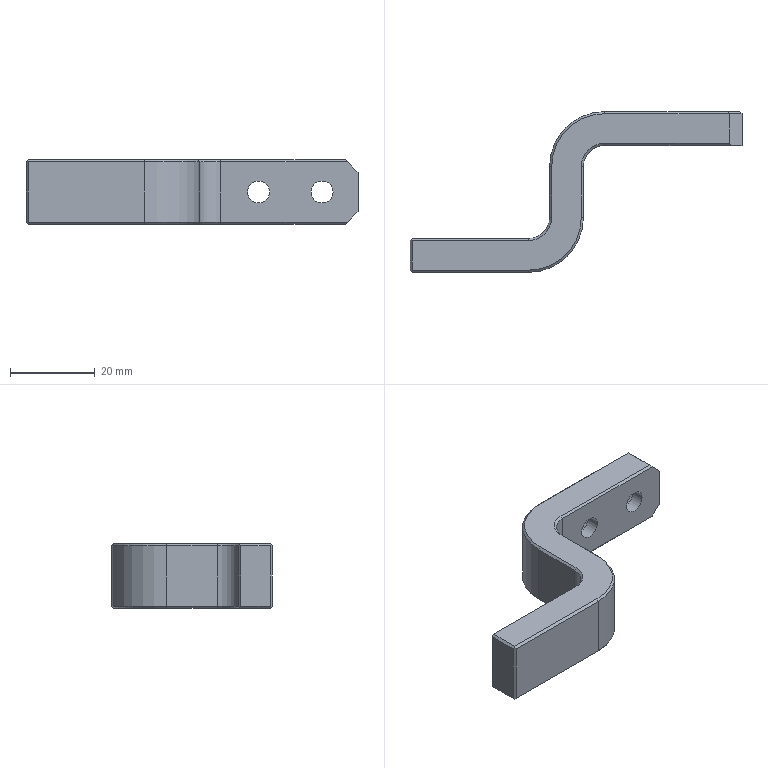Part | Creo | features CURVE 3, DATUM PLANE 3, CHAMFER 2, CUT 2, COORDINATE SYSTEM 1, PROTRUSION 1 | 1 solid | 53 faces | box 78.5 x 38 x 15.3 mm | volume 11414 mm3 | plane 33 | cylinder 12 | cone 8 | commonest cylinder face diameters 5.2 x4 9.2 x4 10 x2 26 x2
STEP:
#1=CARTESIAN_POINT('',(0.,0.,0.));
#2=DIRECTION('',(0.,0.,1.));
#3=DIRECTION('',(1.,0.,0.));
#4=AXIS2_PLACEMENT_3D('',#1,#2,#3);
#5=CARTESIAN_POINT('',(25.5,7.5,-7.65));
#6=VERTEX_POINT('',#5);
#7=CARTESIAN_POINT('',(-4.,7.5,-7.65));
#8=VERTEX_POINT('',#7);
#9=CARTESIAN_POINT('',(25.5,7.5,-7.65));
#10=DIRECTION('',(-1.,0.,0.));
#11=VECTOR('',#10,29.5);
#12=LINE('',#9,#11);
#13=EDGE_CURVE('',#6,#8,#12,.T.);
#14=ORIENTED_EDGE('',*,*,#13,.F.);
#15=CARTESIAN_POINT('',(25.5,14.5,-7.65));
#16=VERTEX_POINT('',#15);
#17=CARTESIAN_POINT('',(25.5,14.5,-7.65));
#18=DIRECTION('',(0.,-1.,0.));
#19=VECTOR('',#18,7.);
#20=LINE('',#17,#19);
#21=EDGE_CURVE('',#16,#6,#20,.T.);
#22=ORIENTED_EDGE('',*,*,#21,.F.);
#23=CARTESIAN_POINT('',(-4.,14.5,-7.65));
#24=VERTEX_POINT('',#23);
#25=CARTESIAN_POINT('',(-4.,14.5,-7.65));
#26=DIRECTION('',(1.,0.,0.));
#27=VECTOR('',#26,29.5);
#28=LINE('',#25,#27);
#29=EDGE_CURVE('',#24,#16,#28,.T.);
#30=ORIENTED_EDGE('',*,*,#29,.F.);
#31=CARTESIAN_POINT('',(-16.5,2.,-7.65));
#32=VERTEX_POINT('',#31);
#33=CARTESIAN_POINT('',(-4.,2.,-7.65));
#34=DIRECTION('',(0.,0.,-1.));
#35=DIRECTION('',(-1.,0.,0.));
#36=AXIS2_PLACEMENT_3D('',#33,#34,#35);
#37=CIRCLE('',#36,12.5);
#38=EDGE_CURVE('',#32,#24,#37,.T.);
#39=ORIENTED_EDGE('',*,*,#38,.F.);
#40=CARTESIAN_POINT('',(-16.5,-10.,-7.65));
#41=VERTEX_POINT('',#40);
#42=CARTESIAN_POINT('',(-16.5,-10.,-7.65));
#43=DIRECTION('',(0.,1.,0.));
#44=VECTOR('',#43,12.);
#45=LINE('',#42,#44);
#46=EDGE_CURVE('',#41,#32,#45,.T.);
#47=ORIENTED_EDGE('',*,*,#46,.F.);
#48=CARTESIAN_POINT('',(-22.,-15.5,-7.65));
#49=VERTEX_POINT('',#48);
#50=CARTESIAN_POINT('',(-22.,-10.,-7.65));
#51=DIRECTION('',(0.,0.,1.));
#52=DIRECTION('',(0.,-1.,0.));
#53=AXIS2_PLACEMENT_3D('',#50,#51,#52);
#54=CIRCLE('',#53,5.5);
#55=EDGE_CURVE('',#49,#41,#54,.T.);
#56=ORIENTED_EDGE('',*,*,#55,.F.);
#57=CARTESIAN_POINT('',(-49.5,-15.5,-7.65));
#58=VERTEX_POINT('',#57);
#59=CARTESIAN_POINT('',(-49.5,-15.5,-7.65));
#60=DIRECTION('',(1.,0.,0.));
#61=VECTOR('',#60,27.5);
#62=LINE('',#59,#61);
#63=EDGE_CURVE('',#58,#49,#62,.T.);
#64=ORIENTED_EDGE('',*,*,#63,.F.);
#65=CARTESIAN_POINT('',(-49.5,-22.5,-7.65));
#66=VERTEX_POINT('',#65);
#67=CARTESIAN_POINT('',(-49.5,-22.5,-7.65));
#68=DIRECTION('',(0.,1.,0.));
#69=VECTOR('',#68,7.);
#70=LINE('',#67,#69);
#71=EDGE_CURVE('',#66,#58,#70,.T.);
#72=ORIENTED_EDGE('',*,*,#71,.F.);
#73=CARTESIAN_POINT('',(-22.,-22.5,-7.65));
#74=VERTEX_POINT('',#73);
#75=CARTESIAN_POINT('',(-22.,-22.5,-7.65));
#76=DIRECTION('',(-1.,0.,0.));
#77=VECTOR('',#76,27.5);
#78=LINE('',#75,#77);
#79=EDGE_CURVE('',#74,#66,#78,.T.);
#80=ORIENTED_EDGE('',*,*,#79,.F.);
#81=CARTESIAN_POINT('',(-9.5,-10.,-7.65));
#82=VERTEX_POINT('',#81);
#83=CARTESIAN_POINT('',(-22.,-10.,-7.65));
#84=DIRECTION('',(0.,0.,-1.));
#85=DIRECTION('',(1.,0.,0.));
#86=AXIS2_PLACEMENT_3D('',#83,#84,#85);
#87=CIRCLE('',#86,12.5);
#88=EDGE_CURVE('',#82,#74,#87,.T.);
#89=ORIENTED_EDGE('',*,*,#88,.F.);
#90=CARTESIAN_POINT('',(-9.5,2.,-7.65));
#91=VERTEX_POINT('',#90);
#92=CARTESIAN_POINT('',(-9.5,2.,-7.65));
#93=DIRECTION('',(0.,-1.,0.));
#94=VECTOR('',#93,12.);
#95=LINE('',#92,#94);
#96=EDGE_CURVE('',#91,#82,#95,.T.);
#97=ORIENTED_EDGE('',*,*,#96,.F.);
#98=CARTESIAN_POINT('',(-4.,2.,-7.65));
#99=DIRECTION('',(0.,0.,1.));
#100=DIRECTION('',(0.,1.,0.));
#101=AXIS2_PLACEMENT_3D('',#98,#99,#100);
#102=CIRCLE('',#101,5.5);
#103=EDGE_CURVE('',#8,#91,#102,.T.);
#104=ORIENTED_EDGE('',*,*,#103,.F.);
#105=EDGE_LOOP('',(#14,#22,#30,#39,#47,#56,#64,#72,#80,#89,#97,#104));
#106=FACE_OUTER_BOUND('',#105,.F.);
#107=CARTESIAN_POINT('',(0.,0.,-7.65));
#108=DIRECTION('',(0.,0.,1.));
#109=DIRECTION('',(1.,0.,0.));
#110=AXIS2_PLACEMENT_3D('',#107,#108,#109);
#111=PLANE('',#110);
#112=ADVANCED_FACE('',(#106),#111,.F.);
#113=CARTESIAN_POINT('',(26.,7.,-7.15));
#114=VERTEX_POINT('',#113);
#115=CARTESIAN_POINT('',(26.,7.,-7.15));
#116=DIRECTION('',(-0.5774,0.5774,-0.5774));
#117=VECTOR('',#116,0.866);
#118=LINE('',#115,#117);
#119=EDGE_CURVE('',#114,#6,#118,.T.);
#120=ORIENTED_EDGE('',*,*,#119,.T.);
#121=ORIENTED_EDGE('',*,*,#13,.T.);
#122=CARTESIAN_POINT('',(-4.,7.,-7.15));
#123=VERTEX_POINT('',#122);
#124=CARTESIAN_POINT('',(-4.,7.5,-7.65));
#125=DIRECTION('',(0.000000027,-0.7071,0.7071));
#126=VECTOR('',#125,0.7071);
#127=LINE('',#124,#126);
#128=EDGE_CURVE('',#8,#123,#127,.T.);
#129=ORIENTED_EDGE('',*,*,#128,.T.);
#130=CARTESIAN_POINT('',(26.,7.,-7.15));
#131=DIRECTION('',(-1.,0.,0.));
#132=VECTOR('',#131,30.);
#133=LINE('',#130,#132);
#134=EDGE_CURVE('',#114,#123,#133,.T.);
#135=ORIENTED_EDGE('',*,*,#134,.F.);
#136=EDGE_LOOP('',(#120,#121,#129,#135));
#137=FACE_OUTER_BOUND('',#136,.F.);
#138=CARTESIAN_POINT('',(10.75,7.25,-7.4));
#139=DIRECTION('',(0.,-0.7071,-0.7071));
#140=DIRECTION('',(0.,-0.7071,0.7071));
#141=AXIS2_PLACEMENT_3D('',#138,#139,#140);
#142=PLANE('',#141);
#143=ADVANCED_FACE('',(#137),#142,.T.);
#144=ORIENTED_EDGE('',*,*,#119,.F.);
#145=CARTESIAN_POINT('',(28.5,7.,-4.65));
#146=VERTEX_POINT('',#145);
#147=CARTESIAN_POINT('',(26.,7.,-7.15));
#148=DIRECTION('',(0.7071,0.,0.7071));
#149=VECTOR('',#148,3.536);
#150=LINE('',#147,#149);
#151=EDGE_CURVE('',#114,#146,#150,.T.);
#152=ORIENTED_EDGE('',*,*,#151,.T.);
#153=CARTESIAN_POINT('',(28.5,14.5,-4.65));
#154=VERTEX_POINT('',#153);
#155=CARTESIAN_POINT('',(28.5,14.5,-4.65));
#156=DIRECTION('',(0.,-1.,0.));
#157=VECTOR('',#156,7.5);
#158=LINE('',#155,#157);
#159=EDGE_CURVE('',#154,#146,#158,.T.);
#160=ORIENTED_EDGE('',*,*,#159,.F.);
#161=CARTESIAN_POINT('',(28.5,14.5,-4.65));
#162=DIRECTION('',(-0.7071,0.,-0.7071));
#163=VECTOR('',#162,4.243);
#164=LINE('',#161,#163);
#165=EDGE_CURVE('',#154,#16,#164,.T.);
#166=ORIENTED_EDGE('',*,*,#165,.T.);
#167=ORIENTED_EDGE('',*,*,#21,.T.);
#168=EDGE_LOOP('',(#144,#152,#160,#166,#167));
#169=FACE_OUTER_BOUND('',#168,.F.);
#170=CARTESIAN_POINT('',(27.,11.,-6.15));
#171=DIRECTION('',(0.7071,0.,-0.7071));
#172=DIRECTION('',(0.7071,0.,0.7071));
#173=AXIS2_PLACEMENT_3D('',#170,#171,#172);
#174=PLANE('',#173);
#175=ADVANCED_FACE('',(#169),#174,.T.);
#176=CARTESIAN_POINT('',(-4.,7.,7.15));
#177=VERTEX_POINT('',#176);
#178=CARTESIAN_POINT('',(26.,7.,7.15));
#179=VERTEX_POINT('',#178);
#180=CARTESIAN_POINT('',(-4.,7.,7.15));
#181=DIRECTION('',(1.,0.,0.));
#182=VECTOR('',#181,30.);
#183=LINE('',#180,#182);
#184=EDGE_CURVE('',#177,#179,#183,.T.);
#185=ORIENTED_EDGE('',*,*,#184,.T.);
#186=CARTESIAN_POINT('',(28.5,7.,4.65));
#187=VERTEX_POINT('',#186);
#188=CARTESIAN_POINT('',(28.5,7.,4.65));
#189=DIRECTION('',(-0.7071,0.,0.7071));
#190=VECTOR('',#189,3.536);
#191=LINE('',#188,#190);
#192=EDGE_CURVE('',#187,#179,#191,.T.);
#193=ORIENTED_EDGE('',*,*,#192,.F.);
#194=CARTESIAN_POINT('',(28.5,7.,-4.65));
#195=DIRECTION('',(0.,0.,1.));
#196=VECTOR('',#195,9.3);
#197=LINE('',#194,#196);
#198=EDGE_CURVE('',#146,#187,#197,.T.);
#199=ORIENTED_EDGE('',*,*,#198,.F.);
#200=ORIENTED_EDGE('',*,*,#151,.F.);
#201=ORIENTED_EDGE('',*,*,#134,.T.);
#202=CARTESIAN_POINT('',(-4.,7.,-7.15));
#203=DIRECTION('',(-0.000000003,0.,1.));
#204=VECTOR('',#203,14.3);
#205=LINE('',#202,#204);
#206=EDGE_CURVE('',#123,#177,#205,.T.);
#207=ORIENTED_EDGE('',*,*,#206,.T.);
#208=EDGE_LOOP('',(#185,#193,#199,#200,#201,#207));
#209=FACE_OUTER_BOUND('',#208,.F.);
#210=CARTESIAN_POINT('',(7.6,7.,0.));
#211=VERTEX_POINT('',#210);
#212=CARTESIAN_POINT('',(2.4,7.,0.));
#213=VERTEX_POINT('',#212);
#214=CARTESIAN_POINT('',(5.,7.,0.));
#215=DIRECTION('',(0.,1.,0.));
#216=DIRECTION('',(1.,0.,0.));
#217=AXIS2_PLACEMENT_3D('',#214,#215,#216);
#218=CIRCLE('',#217,2.6);
#219=EDGE_CURVE('',#211,#213,#218,.T.);
#220=ORIENTED_EDGE('',*,*,#219,.F.);
#221=CARTESIAN_POINT('',(5.,7.,0.));
#222=DIRECTION('',(0.,1.,0.));
#223=DIRECTION('',(-1.,0.,0.));
#224=AXIS2_PLACEMENT_3D('',#221,#222,#223);
#225=CIRCLE('',#224,2.6);
#226=EDGE_CURVE('',#213,#211,#225,.T.);
#227=ORIENTED_EDGE('',*,*,#226,.F.);
#228=EDGE_LOOP('',(#220,#227));
#229=FACE_BOUND('',#228,.F.);
#230=CARTESIAN_POINT('',(22.6,7.,0.));
#231=VERTEX_POINT('',#230);
#232=CARTESIAN_POINT('',(17.4,7.,0.));
#233=VERTEX_POINT('',#232);
#234=CARTESIAN_POINT('',(20.,7.,0.));
#235=DIRECTION('',(0.,1.,0.));
#236=DIRECTION('',(1.,0.,0.));
#237=AXIS2_PLACEMENT_3D('',#234,#235,#236);
#238=CIRCLE('',#237,2.6);
#239=EDGE_CURVE('',#231,#233,#238,.T.);
#240=ORIENTED_EDGE('',*,*,#239,.F.);
#241=CARTESIAN_POINT('',(20.,7.,0.));
#242=DIRECTION('',(0.,1.,0.));
#243=DIRECTION('',(-1.,0.,0.));
#244=AXIS2_PLACEMENT_3D('',#241,#242,#243);
#245=CIRCLE('',#244,2.6);
#246=EDGE_CURVE('',#233,#231,#245,.T.);
#247=ORIENTED_EDGE('',*,*,#246,.F.);
#248=EDGE_LOOP('',(#240,#247));
#249=FACE_BOUND('',#248,.F.);
#250=CARTESIAN_POINT('',(-4.,7.,-7.65));
#251=DIRECTION('',(0.,-1.,0.));
#252=DIRECTION('',(1.,0.,0.));
#253=AXIS2_PLACEMENT_3D('',#250,#251,#252);
#254=PLANE('',#253);
#255=ADVANCED_FACE('',(#209,#229,#249),#254,.T.);
#256=CARTESIAN_POINT('',(22.6,10.,0.));
#257=VERTEX_POINT('',#256);
#258=CARTESIAN_POINT('',(17.4,10.,0.));
#259=VERTEX_POINT('',#258);
#260=CARTESIAN_POINT('',(20.,10.,0.));
#261=DIRECTION('',(0.,1.,0.));
#262=DIRECTION('',(1.,0.,0.));
#263=AXIS2_PLACEMENT_3D('',#260,#261,#262);
#264=CIRCLE('',#263,2.6);
#265=EDGE_CURVE('',#257,#259,#264,.T.);
#266=ORIENTED_EDGE('',*,*,#265,.F.);
#267=CARTESIAN_POINT('',(22.6,10.,0.));
#268=DIRECTION('',(0.,-1.,0.));
#269=VECTOR('',#268,3.);
#270=LINE('',#267,#269);
#271=EDGE_CURVE('',#257,#231,#270,.T.);
#272=ORIENTED_EDGE('',*,*,#271,.T.);
#273=ORIENTED_EDGE('',*,*,#239,.T.);
#274=CARTESIAN_POINT('',(17.4,10.,0.));
#275=DIRECTION('',(0.,-1.,0.));
#276=VECTOR('',#275,3.);
#277=LINE('',#274,#276);
#278=EDGE_CURVE('',#259,#233,#277,.T.);
#279=ORIENTED_EDGE('',*,*,#278,.F.);
#280=EDGE_LOOP('',(#266,#272,#273,#279));
#281=FACE_OUTER_BOUND('',#280,.F.);
#282=CARTESIAN_POINT('',(20.,15.,0.));
#283=DIRECTION('',(0.,1.,0.));
#284=DIRECTION('',(1.,0.,0.));
#285=AXIS2_PLACEMENT_3D('',#282,#283,#284);
#286=CYLINDRICAL_SURFACE('',#285,2.6);
#287=ADVANCED_FACE('',(#281),#286,.F.);
#288=CARTESIAN_POINT('',(24.6,10.,0.));
#289=VERTEX_POINT('',#288);
#290=CARTESIAN_POINT('',(15.4,10.,0.));
#291=VERTEX_POINT('',#290);
#292=CARTESIAN_POINT('',(20.,10.,0.));
#293=DIRECTION('',(0.,1.,0.));
#294=DIRECTION('',(1.,0.,0.));
#295=AXIS2_PLACEMENT_3D('',#292,#293,#294);
#296=CIRCLE('',#295,4.6);
#297=EDGE_CURVE('',#289,#291,#296,.T.);
#298=ORIENTED_EDGE('',*,*,#297,.F.);
#299=CARTESIAN_POINT('',(20.,10.,0.));
#300=DIRECTION('',(0.,1.,0.));
#301=DIRECTION('',(-1.,0.,0.));
#302=AXIS2_PLACEMENT_3D('',#299,#300,#301);
#303=CIRCLE('',#302,4.6);
#304=EDGE_CURVE('',#291,#289,#303,.T.);
#305=ORIENTED_EDGE('',*,*,#304,.F.);
#306=EDGE_LOOP('',(#298,#305));
#307=FACE_OUTER_BOUND('',#306,.F.);
#308=ORIENTED_EDGE('',*,*,#265,.T.);
#309=CARTESIAN_POINT('',(20.,10.,0.));
#310=DIRECTION('',(0.,1.,0.));
#311=DIRECTION('',(-1.,0.,0.));
#312=AXIS2_PLACEMENT_3D('',#309,#310,#311);
#313=CIRCLE('',#312,2.6);
#314=EDGE_CURVE('',#259,#257,#313,.T.);
#315=ORIENTED_EDGE('',*,*,#314,.T.);
#316=EDGE_LOOP('',(#308,#315));
#317=FACE_BOUND('',#316,.F.);
#318=CARTESIAN_POINT('',(0.,10.,-7.65));
#319=DIRECTION('',(0.,1.,0.));
#320=DIRECTION('',(1.,0.,0.));
#321=AXIS2_PLACEMENT_3D('',#318,#319,#320);
#322=PLANE('',#321);
#323=ADVANCED_FACE('',(#307,#317),#322,.T.);
#324=CARTESIAN_POINT('',(9.6,10.,0.));
#325=VERTEX_POINT('',#324);
#326=CARTESIAN_POINT('',(0.4,10.,0.));
#327=VERTEX_POINT('',#326);
#328=CARTESIAN_POINT('',(5.,10.,0.));
#329=DIRECTION('',(0.,1.,0.));
#330=DIRECTION('',(1.,0.,0.));
#331=AXIS2_PLACEMENT_3D('',#328,#329,#330);
#332=CIRCLE('',#331,4.6);
#333=EDGE_CURVE('',#325,#327,#332,.T.);
#334=ORIENTED_EDGE('',*,*,#333,.F.);
#335=CARTESIAN_POINT('',(5.,10.,0.));
#336=DIRECTION('',(0.,1.,0.));
#337=DIRECTION('',(-1.,0.,0.));
#338=AXIS2_PLACEMENT_3D('',#335,#336,#337);
#339=CIRCLE('',#338,4.6);
#340=EDGE_CURVE('',#327,#325,#339,.T.);
#341=ORIENTED_EDGE('',*,*,#340,.F.);
#342=EDGE_LOOP('',(#334,#341));
#343=FACE_OUTER_BOUND('',#342,.F.);
#344=CARTESIAN_POINT('',(7.6,10.,0.));
#345=VERTEX_POINT('',#344);
#346=CARTESIAN_POINT('',(2.4,10.,0.));
#347=VERTEX_POINT('',#346);
#348=CARTESIAN_POINT('',(5.,10.,0.));
#349=DIRECTION('',(0.,1.,0.));
#350=DIRECTION('',(1.,0.,0.));
#351=AXIS2_PLACEMENT_3D('',#348,#349,#350);
#352=CIRCLE('',#351,2.6);
#353=EDGE_CURVE('',#345,#347,#352,.T.);
#354=ORIENTED_EDGE('',*,*,#353,.T.);
#355=CARTESIAN_POINT('',(5.,10.,0.));
#356=DIRECTION('',(0.,1.,0.));
#357=DIRECTION('',(-1.,0.,0.));
#358=AXIS2_PLACEMENT_3D('',#355,#356,#357);
#359=CIRCLE('',#358,2.6);
#360=EDGE_CURVE('',#347,#345,#359,.T.);
#361=ORIENTED_EDGE('',*,*,#360,.T.);
#362=EDGE_LOOP('',(#354,#361));
#363=FACE_BOUND('',#362,.F.);
#364=CARTESIAN_POINT('',(0.,10.,-7.65));
#365=DIRECTION('',(0.,1.,0.));
#366=DIRECTION('',(1.,0.,0.));
#367=AXIS2_PLACEMENT_3D('',#364,#365,#366);
#368=PLANE('',#367);
#369=ADVANCED_FACE('',(#343,#363),#368,.T.);
#370=CARTESIAN_POINT('',(24.6,15.,0.));
#371=VERTEX_POINT('',#370);
#372=CARTESIAN_POINT('',(15.4,15.,0.));
#373=VERTEX_POINT('',#372);
#374=CARTESIAN_POINT('',(20.,15.,0.));
#375=DIRECTION('',(0.,1.,0.));
#376=DIRECTION('',(1.,0.,0.));
#377=AXIS2_PLACEMENT_3D('',#374,#375,#376);
#378=CIRCLE('',#377,4.6);
#379=EDGE_CURVE('',#371,#373,#378,.T.);
#380=ORIENTED_EDGE('',*,*,#379,.F.);
#381=CARTESIAN_POINT('',(24.6,15.,0.));
#382=DIRECTION('',(0.,-1.,0.));
#383=VECTOR('',#382,5.);
#384=LINE('',#381,#383);
#385=EDGE_CURVE('',#371,#289,#384,.T.);
#386=ORIENTED_EDGE('',*,*,#385,.T.);
#387=ORIENTED_EDGE('',*,*,#297,.T.);
#388=CARTESIAN_POINT('',(15.4,15.,0.));
#389=DIRECTION('',(0.,-1.,0.));
#390=VECTOR('',#389,5.);
#391=LINE('',#388,#390);
#392=EDGE_CURVE('',#373,#291,#391,.T.);
#393=ORIENTED_EDGE('',*,*,#392,.F.);
#394=EDGE_LOOP('',(#380,#386,#387,#393));
#395=FACE_OUTER_BOUND('',#394,.F.);
#396=CARTESIAN_POINT('',(20.,15.,0.));
#397=DIRECTION('',(0.,1.,0.));
#398=DIRECTION('',(1.,0.,0.));
#399=AXIS2_PLACEMENT_3D('',#396,#397,#398);
#400=CYLINDRICAL_SURFACE('',#399,4.6);
#401=ADVANCED_FACE('',(#395),#400,.F.);
#402=CARTESIAN_POINT('',(-4.,15.,-7.15));
#403=VERTEX_POINT('',#402);
#404=CARTESIAN_POINT('',(25.293,15.,-7.15));
#405=VERTEX_POINT('',#404);
#406=CARTESIAN_POINT('',(-4.,15.,-7.15));
#407=DIRECTION('',(1.,0.,0.));
#408=VECTOR('',#407,29.293);
#409=LINE('',#406,#408);
#410=EDGE_CURVE('',#403,#405,#409,.T.);
#411=ORIENTED_EDGE('',*,*,#410,.T.);
#412=CARTESIAN_POINT('',(28.,15.,-4.443));
#413=VERTEX_POINT('',#412);
#414=CARTESIAN_POINT('',(28.,15.,-4.443));
#415=DIRECTION('',(-0.7071,0.,-0.7071));
#416=VECTOR('',#415,3.828);
#417=LINE('',#414,#416);
#418=EDGE_CURVE('',#413,#405,#417,.T.);
#419=ORIENTED_EDGE('',*,*,#418,.F.);
#420=CARTESIAN_POINT('',(28.,15.,4.443));
#421=VERTEX_POINT('',#420);
#422=CARTESIAN_POINT('',(28.,15.,4.443));
#423=DIRECTION('',(0.,0.,-1.));
#424=VECTOR('',#423,8.886);
#425=LINE('',#422,#424);
#426=EDGE_CURVE('',#421,#413,#425,.T.);
#427=ORIENTED_EDGE('',*,*,#426,.F.);
#428=CARTESIAN_POINT('',(25.293,15.,7.15));
#429=VERTEX_POINT('',#428);
#430=CARTESIAN_POINT('',(25.293,15.,7.15));
#431=DIRECTION('',(0.7071,0.,-0.7071));
#432=VECTOR('',#431,3.828);
#433=LINE('',#430,#432);
#434=EDGE_CURVE('',#429,#421,#433,.T.);
#435=ORIENTED_EDGE('',*,*,#434,.F.);
#436=CARTESIAN_POINT('',(-4.,15.,7.15));
#437=VERTEX_POINT('',#436);
#438=CARTESIAN_POINT('',(25.293,15.,7.15));
#439=DIRECTION('',(-1.,0.,0.));
#440=VECTOR('',#439,29.293);
#441=LINE('',#438,#440);
#442=EDGE_CURVE('',#429,#437,#441,.T.);
#443=ORIENTED_EDGE('',*,*,#442,.T.);
#444=CARTESIAN_POINT('',(-4.,15.,-7.15));
#445=DIRECTION('',(0.000000002,0.,1.));
#446=VECTOR('',#445,14.3);
#447=LINE('',#444,#446);
#448=EDGE_CURVE('',#403,#437,#447,.T.);
#449=ORIENTED_EDGE('',*,*,#448,.F.);
#450=EDGE_LOOP('',(#411,#419,#427,#435,#443,#449));
#451=FACE_OUTER_BOUND('',#450,.F.);
#452=CARTESIAN_POINT('',(9.6,15.,0.));
#453=VERTEX_POINT('',#452);
#454=CARTESIAN_POINT('',(0.4,15.,0.));
#455=VERTEX_POINT('',#454);
#456=CARTESIAN_POINT('',(5.,15.,0.));
#457=DIRECTION('',(0.,1.,0.));
#458=DIRECTION('',(1.,0.,0.));
#459=AXIS2_PLACEMENT_3D('',#456,#457,#458);
#460=CIRCLE('',#459,4.6);
#461=EDGE_CURVE('',#453,#455,#460,.T.);
#462=ORIENTED_EDGE('',*,*,#461,.T.);
#463=CARTESIAN_POINT('',(5.,15.,0.));
#464=DIRECTION('',(0.,1.,0.));
#465=DIRECTION('',(-1.,0.,0.));
#466=AXIS2_PLACEMENT_3D('',#463,#464,#465);
#467=CIRCLE('',#466,4.6);
#468=EDGE_CURVE('',#455,#453,#467,.T.);
#469=ORIENTED_EDGE('',*,*,#468,.T.);
#470=EDGE_LOOP('',(#462,#469));
#471=FACE_BOUND('',#470,.F.);
#472=ORIENTED_EDGE('',*,*,#379,.T.);
#473=CARTESIAN_POINT('',(20.,15.,0.));
#474=DIRECTION('',(0.,1.,0.));
#475=DIRECTION('',(-1.,0.,0.));
#476=AXIS2_PLACEMENT_3D('',#473,#474,#475);
#477=CIRCLE('',#476,4.6);
#478=EDGE_CURVE('',#373,#371,#477,.T.);
#479=ORIENTED_EDGE('',*,*,#478,.T.);
#480=EDGE_LOOP('',(#472,#479));
#481=FACE_BOUND('',#480,.F.);
#482=CARTESIAN_POINT('',(28.5,15.,-7.65));
#483=DIRECTION('',(0.,1.,0.));
#484=DIRECTION('',(-1.,0.,0.));
#485=AXIS2_PLACEMENT_3D('',#482,#483,#484);
#486=PLANE('',#485);
#487=ADVANCED_FACE('',(#451,#471,#481),#486,.T.);
#488=ORIENTED_EDGE('',*,*,#478,.F.);
#489=ORIENTED_EDGE('',*,*,#392,.T.);
#490=ORIENTED_EDGE('',*,*,#304,.T.);
#491=ORIENTED_EDGE('',*,*,#385,.F.);
#492=EDGE_LOOP('',(#488,#489,#490,#491));
#493=FACE_OUTER_BOUND('',#492,.F.);
#494=CARTESIAN_POINT('',(20.,15.,0.));
#495=DIRECTION('',(0.,1.,0.));
#496=DIRECTION('',(1.,0.,0.));
#497=AXIS2_PLACEMENT_3D('',#494,#495,#496);
#498=CYLINDRICAL_SURFACE('',#497,4.6);
#499=ADVANCED_FACE('',(#493),#498,.F.);
#500=ORIENTED_EDGE('',*,*,#461,.F.);
#501=CARTESIAN_POINT('',(9.6,15.,0.));
#502=DIRECTION('',(0.,-1.,0.));
#503=VECTOR('',#502,5.);
#504=LINE('',#501,#503);
#505=EDGE_CURVE('',#453,#325,#504,.T.);
#506=ORIENTED_EDGE('',*,*,#505,.T.);
#507=ORIENTED_EDGE('',*,*,#333,.T.);
#508=CARTESIAN_POINT('',(0.4,15.,0.));
#509=DIRECTION('',(0.,-1.,0.));
#510=VECTOR('',#509,5.);
#511=LINE('',#508,#510);
#512=EDGE_CURVE('',#455,#327,#511,.T.);
#513=ORIENTED_EDGE('',*,*,#512,.F.);
#514=EDGE_LOOP('',(#500,#506,#507,#513));
#515=FACE_OUTER_BOUND('',#514,.F.);
#516=CARTESIAN_POINT('',(5.,15.,0.));
#517=DIRECTION('',(0.,1.,0.));
#518=DIRECTION('',(1.,0.,0.));
#519=AXIS2_PLACEMENT_3D('',#516,#517,#518);
#520=CYLINDRICAL_SURFACE('',#519,4.6);
#521=ADVANCED_FACE('',(#515),#520,.F.);
#522=ORIENTED_EDGE('',*,*,#468,.F.);
#523=ORIENTED_EDGE('',*,*,#512,.T.);
#524=ORIENTED_EDGE('',*,*,#340,.T.);
#525=ORIENTED_EDGE('',*,*,#505,.F.);
#526=EDGE_LOOP('',(#522,#523,#524,#525));
#527=FACE_OUTER_BOUND('',#526,.F.);
#528=CARTESIAN_POINT('',(5.,15.,0.));
#529=DIRECTION('',(0.,1.,0.));
#530=DIRECTION('',(1.,0.,0.));
#531=AXIS2_PLACEMENT_3D('',#528,#529,#530);
#532=CYLINDRICAL_SURFACE('',#531,4.6);
#533=ADVANCED_FACE('',(#527),#532,.F.);
#534=ORIENTED_EDGE('',*,*,#410,.F.);
#535=CARTESIAN_POINT('',(-4.,14.5,-7.65));
#536=DIRECTION('',(-0.000000009,0.7071,0.7071));
#537=VECTOR('',#536,0.7071);
#538=LINE('',#535,#537);
#539=EDGE_CURVE('',#24,#403,#538,.T.);
#540=ORIENTED_EDGE('',*,*,#539,.F.);
#541=ORIENTED_EDGE('',*,*,#29,.T.);
#542=CARTESIAN_POINT('',(25.5,14.5,-7.65));
#543=DIRECTION('',(-0.2811,0.6786,0.6786));
#544=VECTOR('',#543,0.7368);
#545=LINE('',#542,#544);
#546=EDGE_CURVE('',#16,#405,#545,.T.);
#547=ORIENTED_EDGE('',*,*,#546,.T.);
#548=EDGE_LOOP('',(#534,#540,#541,#547));
#549=FACE_OUTER_BOUND('',#548,.F.);
#550=CARTESIAN_POINT('',(10.75,14.75,-7.4));
#551=DIRECTION('',(0.,0.7071,-0.7071));
#552=DIRECTION('',(0.,0.7071,0.7071));
#553=AXIS2_PLACEMENT_3D('',#550,#551,#552);
#554=PLANE('',#553);
#555=ADVANCED_FACE('',(#549),#554,.T.);
#556=ORIENTED_EDGE('',*,*,#38,.T.);
#557=ORIENTED_EDGE('',*,*,#539,.T.);
#558=CARTESIAN_POINT('',(-17.,2.,-7.15));
#559=VERTEX_POINT('',#558);
#560=CARTESIAN_POINT('',(-4.,2.,-7.15));
#561=DIRECTION('',(0.,0.,-1.));
#562=DIRECTION('',(-1.,0.,0.));
#563=AXIS2_PLACEMENT_3D('',#560,#561,#562);
#564=CIRCLE('',#563,13.);
#565=EDGE_CURVE('',#559,#403,#564,.T.);
#566=ORIENTED_EDGE('',*,*,#565,.F.);
#567=CARTESIAN_POINT('',(-16.5,2.,-7.65));
#568=DIRECTION('',(-0.7071,0.00000001,0.7071));
#569=VECTOR('',#568,0.7071);
#570=LINE('',#567,#569);
#571=EDGE_CURVE('',#32,#559,#570,.T.);
#572=ORIENTED_EDGE('',*,*,#571,.F.);
#573=EDGE_LOOP('',(#556,#557,#566,#572));
#574=FACE_OUTER_BOUND('',#573,.F.);
#575=CARTESIAN_POINT('',(-4.,2.,-7.4));
#576=DIRECTION('',(0.,0.,1.));
#577=DIRECTION('',(0.,-1.,0.));
#578=AXIS2_PLACEMENT_3D('',#575,#576,#577);
#579=CONICAL_SURFACE('',#578,12.75,45.);
#580=ADVANCED_FACE('',(#574),#579,.T.);
#581=ORIENTED_EDGE('',*,*,#565,.T.);
#582=ORIENTED_EDGE('',*,*,#448,.T.);
#583=CARTESIAN_POINT('',(-17.,2.,7.15));
#584=VERTEX_POINT('',#583);
#585=CARTESIAN_POINT('',(-4.,2.,7.15));
#586=DIRECTION('',(0.,0.,1.));
#587=DIRECTION('',(0.,1.,0.));
#588=AXIS2_PLACEMENT_3D('',#585,#586,#587);
#589=CIRCLE('',#588,13.);
#590=EDGE_CURVE('',#437,#584,#589,.T.);
#591=ORIENTED_EDGE('',*,*,#590,.T.);
#592=CARTESIAN_POINT('',(-17.,2.,-7.15));
#593=DIRECTION('',(0.,0.,1.));
#594=VECTOR('',#593,14.3);
#595=LINE('',#592,#594);
#596=EDGE_CURVE('',#559,#584,#595,.T.);
#597=ORIENTED_EDGE('',*,*,#596,.F.);
#598=EDGE_LOOP('',(#581,#582,#591,#597));
#599=FACE_OUTER_BOUND('',#598,.F.);
#600=CARTESIAN_POINT('',(-4.,2.,-7.65));
#601=DIRECTION('',(0.,0.,1.));
#602=DIRECTION('',(1.,0.,0.));
#603=AXIS2_PLACEMENT_3D('',#600,#601,#602);
#604=CYLINDRICAL_SURFACE('',#603,13.);
#605=ADVANCED_FACE('',(#599),#604,.T.);
#606=CARTESIAN_POINT('',(-4.,14.5,7.65));
#607=VERTEX_POINT('',#606);
#608=CARTESIAN_POINT('',(-16.5,2.,7.65));
#609=VERTEX_POINT('',#608);
#610=CARTESIAN_POINT('',(-4.,2.,7.65));
#611=DIRECTION('',(0.,0.,1.));
#612=DIRECTION('',(0.,1.,0.));
#613=AXIS2_PLACEMENT_3D('',#610,#611,#612);
#614=CIRCLE('',#613,12.5);
#615=EDGE_CURVE('',#607,#609,#614,.T.);
#616=ORIENTED_EDGE('',*,*,#615,.T.);
#617=CARTESIAN_POINT('',(-16.5,2.,7.65));
#618=DIRECTION('',(-0.7071,0.00000001,-0.7071));
#619=VECTOR('',#618,0.7071);
#620=LINE('',#617,#619);
#621=EDGE_CURVE('',#609,#584,#620,.T.);
#622=ORIENTED_EDGE('',*,*,#621,.T.);
#623=ORIENTED_EDGE('',*,*,#590,.F.);
#624=CARTESIAN_POINT('',(-4.,14.5,7.65));
#625=DIRECTION('',(0.000000023,0.7071,-0.7071));
#626=VECTOR('',#625,0.7071);
#627=LINE('',#624,#626);
#628=EDGE_CURVE('',#607,#437,#627,.T.);
#629=ORIENTED_EDGE('',*,*,#628,.F.);
#630=EDGE_LOOP('',(#616,#622,#623,#629));
#631=FACE_OUTER_BOUND('',#630,.F.);
#632=CARTESIAN_POINT('',(-4.,2.,7.4));
#633=DIRECTION('',(0.,0.,-1.));
#634=DIRECTION('',(0.,-1.,0.));
#635=AXIS2_PLACEMENT_3D('',#632,#633,#634);
#636=CONICAL_SURFACE('',#635,12.75,45.);
#637=ADVANCED_FACE('',(#631),#636,.T.);
#638=CARTESIAN_POINT('',(-49.5,-15.5,7.65));
#639=VERTEX_POINT('',#638);
#640=CARTESIAN_POINT('',(-49.5,-22.5,7.65));
#641=VERTEX_POINT('',#640);
#642=CARTESIAN_POINT('',(-49.5,-15.5,7.65));
#643=DIRECTION('',(0.,-1.,0.));
#644=VECTOR('',#643,7.);
#645=LINE('',#642,#644);
#646=EDGE_CURVE('',#639,#641,#645,.T.);
#647=ORIENTED_EDGE('',*,*,#646,.F.);
#648=CARTESIAN_POINT('',(-22.,-15.5,7.65));
#649=VERTEX_POINT('',#648);
#650=CARTESIAN_POINT('',(-22.,-15.5,7.65));
#651=DIRECTION('',(-1.,0.,0.));
#652=VECTOR('',#651,27.5);
#653=LINE('',#650,#652);
#654=EDGE_CURVE('',#649,#639,#653,.T.);
#655=ORIENTED_EDGE('',*,*,#654,.F.);
#656=CARTESIAN_POINT('',(-16.5,-10.,7.65));
#657=VERTEX_POINT('',#656);
#658=CARTESIAN_POINT('',(-22.,-10.,7.65));
#659=DIRECTION('',(0.,0.,-1.));
#660=DIRECTION('',(1.,0.,0.));
#661=AXIS2_PLACEMENT_3D('',#658,#659,#660);
#662=CIRCLE('',#661,5.5);
#663=EDGE_CURVE('',#657,#649,#662,.T.);
#664=ORIENTED_EDGE('',*,*,#663,.F.);
#665=CARTESIAN_POINT('',(-16.5,2.,7.65));
#666=DIRECTION('',(0.,-1.,0.));
#667=VECTOR('',#666,12.);
#668=LINE('',#665,#667);
#669=EDGE_CURVE('',#609,#657,#668,.T.);
#670=ORIENTED_EDGE('',*,*,#669,.F.);
#671=ORIENTED_EDGE('',*,*,#615,.F.);
#672=CARTESIAN_POINT('',(25.5,14.5,7.65));
#673=VERTEX_POINT('',#672);
#674=CARTESIAN_POINT('',(25.5,14.5,7.65));
#675=DIRECTION('',(-1.,0.,0.));
#676=VECTOR('',#675,29.5);
#677=LINE('',#674,#676);
#678=EDGE_CURVE('',#673,#607,#677,.T.);
#679=ORIENTED_EDGE('',*,*,#678,.F.);
#680=CARTESIAN_POINT('',(25.5,7.5,7.65));
#681=VERTEX_POINT('',#680);
#682=CARTESIAN_POINT('',(25.5,7.5,7.65));
#683=DIRECTION('',(0.,1.,0.));
#684=VECTOR('',#683,7.);
#685=LINE('',#682,#684);
#686=EDGE_CURVE('',#681,#673,#685,.T.);
#687=ORIENTED_EDGE('',*,*,#686,.F.);
#688=CARTESIAN_POINT('',(-4.,7.5,7.65));
#689=VERTEX_POINT('',#688);
#690=CARTESIAN_POINT('',(-4.,7.5,7.65));
#691=DIRECTION('',(1.,0.,0.));
#692=VECTOR('',#691,29.5);
#693=LINE('',#690,#692);
#694=EDGE_CURVE('',#689,#681,#693,.T.);
#695=ORIENTED_EDGE('',*,*,#694,.F.);
#696=CARTESIAN_POINT('',(-9.5,2.,7.65));
#697=VERTEX_POINT('',#696);
#698=CARTESIAN_POINT('',(-4.,2.,7.65));
#699=DIRECTION('',(0.,0.,-1.));
#700=DIRECTION('',(-1.,0.,0.));
#701=AXIS2_PLACEMENT_3D('',#698,#699,#700);
#702=CIRCLE('',#701,5.5);
#703=EDGE_CURVE('',#697,#689,#702,.T.);
#704=ORIENTED_EDGE('',*,*,#703,.F.);
#705=CARTESIAN_POINT('',(-9.5,-10.,7.65));
#706=VERTEX_POINT('',#705);
#707=CARTESIAN_POINT('',(-9.5,-10.,7.65));
#708=DIRECTION('',(0.,1.,0.));
#709=VECTOR('',#708,12.);
#710=LINE('',#707,#709);
#711=EDGE_CURVE('',#706,#697,#710,.T.);
#712=ORIENTED_EDGE('',*,*,#711,.F.);
#713=CARTESIAN_POINT('',(-22.,-22.5,7.65));
#714=VERTEX_POINT('',#713);
#715=CARTESIAN_POINT('',(-22.,-10.,7.65));
#716=DIRECTION('',(0.,0.,1.));
#717=DIRECTION('',(0.,-1.,0.));
#718=AXIS2_PLACEMENT_3D('',#715,#716,#717);
#719=CIRCLE('',#718,12.5);
#720=EDGE_CURVE('',#714,#706,#719,.T.);
#721=ORIENTED_EDGE('',*,*,#720,.F.);
#722=CARTESIAN_POINT('',(-49.5,-22.5,7.65));
#723=DIRECTION('',(1.,0.,0.));
#724=VECTOR('',#723,27.5);
#725=LINE('',#722,#724);
#726=EDGE_CURVE('',#641,#714,#725,.T.);
#727=ORIENTED_EDGE('',*,*,#726,.F.);
#728=EDGE_LOOP('',(#647,#655,#664,#670,#671,#679,#687,#695,#704,#712,#721,#727));
#729=FACE_OUTER_BOUND('',#728,.F.);
#730=CARTESIAN_POINT('',(0.,0.,7.65));
#731=DIRECTION('',(0.,0.,1.));
#732=DIRECTION('',(1.,0.,0.));
#733=AXIS2_PLACEMENT_3D('',#730,#731,#732);
#734=PLANE('',#733);
#735=ADVANCED_FACE('',(#729),#734,.T.);
#736=CARTESIAN_POINT('',(-50.,-15.5,7.15));
#737=VERTEX_POINT('',#736);
#738=CARTESIAN_POINT('',(-50.,-22.5,7.15));
#739=VERTEX_POINT('',#738);
#740=CARTESIAN_POINT('',(-50.,-15.5,7.15));
#741=DIRECTION('',(0.,-1.,0.));
#742=VECTOR('',#741,7.);
#743=LINE('',#740,#742);
#744=EDGE_CURVE('',#737,#739,#743,.T.);
#745=ORIENTED_EDGE('',*,*,#744,.F.);
#746=CARTESIAN_POINT('',(-49.75,-15.25,7.4));
#747=VERTEX_POINT('',#746);
#748=CARTESIAN_POINT('',(-50.,-15.5,7.15));
#749=DIRECTION('',(0.5774,0.5774,0.5774));
#750=VECTOR('',#749,0.433);
#751=LINE('',#748,#750);
#752=EDGE_CURVE('',#737,#747,#751,.T.);
#753=ORIENTED_EDGE('',*,*,#752,.T.);
#754=CARTESIAN_POINT('',(-49.5,-15.5,7.65));
#755=DIRECTION('',(-0.5774,0.5774,-0.5774));
#756=VECTOR('',#755,0.433);
#757=LINE('',#754,#756);
#758=EDGE_CURVE('',#639,#747,#757,.T.);
#759=ORIENTED_EDGE('',*,*,#758,.F.);
#760=ORIENTED_EDGE('',*,*,#646,.T.);
#761=CARTESIAN_POINT('',(-49.75,-22.75,7.4));
#762=VERTEX_POINT('',#761);
#763=CARTESIAN_POINT('',(-49.5,-22.5,7.65));
#764=DIRECTION('',(-0.5774,-0.5774,-0.5774));
#765=VECTOR('',#764,0.433);
#766=LINE('',#763,#765);
#767=EDGE_CURVE('',#641,#762,#766,.T.);
#768=ORIENTED_EDGE('',*,*,#767,.T.);
#769=CARTESIAN_POINT('',(-49.75,-22.75,7.4));
#770=DIRECTION('',(-0.5774,0.5774,-0.5774));
#771=VECTOR('',#770,0.433);
#772=LINE('',#769,#771);
#773=EDGE_CURVE('',#762,#739,#772,.T.);
#774=ORIENTED_EDGE('',*,*,#773,.T.);
#775=EDGE_LOOP('',(#745,#753,#759,#760,#768,#774));
#776=FACE_OUTER_BOUND('',#775,.F.);
#777=CARTESIAN_POINT('',(-49.75,-19.,7.4));
#778=DIRECTION('',(-0.7071,0.,0.7071));
#779=DIRECTION('',(-0.7071,0.,-0.7071));
#780=AXIS2_PLACEMENT_3D('',#777,#778,#779);
#781=PLANE('',#780);
#782=ADVANCED_FACE('',(#776),#781,.T.);
#783=CARTESIAN_POINT('',(-50.,-15.5,-7.15));
#784=VERTEX_POINT('',#783);
#785=CARTESIAN_POINT('',(-50.,-15.5,7.15));
#786=DIRECTION('',(0.,0.,-1.));
#787=VECTOR('',#786,14.3);
#788=LINE('',#785,#787);
#789=EDGE_CURVE('',#737,#784,#788,.T.);
#790=ORIENTED_EDGE('',*,*,#789,.F.);
#791=ORIENTED_EDGE('',*,*,#744,.T.);
#792=CARTESIAN_POINT('',(-50.,-22.5,-7.15));
#793=VERTEX_POINT('',#792);
#794=CARTESIAN_POINT('',(-50.,-22.5,7.15));
#795=DIRECTION('',(0.,0.,-1.));
#796=VECTOR('',#795,14.3);
#797=LINE('',#794,#796);
#798=EDGE_CURVE('',#739,#793,#797,.T.);
#799=ORIENTED_EDGE('',*,*,#798,.T.);
#800=CARTESIAN_POINT('',(-50.,-22.5,-7.15));
#801=DIRECTION('',(0.,1.,0.));
#802=VECTOR('',#801,7.);
#803=LINE('',#800,#802);
#804=EDGE_CURVE('',#793,#784,#803,.T.);
#805=ORIENTED_EDGE('',*,*,#804,.T.);
#806=EDGE_LOOP('',(#790,#791,#799,#805));
#807=FACE_OUTER_BOUND('',#806,.F.);
#808=CARTESIAN_POINT('',(-50.,-15.,-7.65));
#809=DIRECTION('',(-1.,0.,0.));
#810=DIRECTION('',(0.,-1.,0.));
#811=AXIS2_PLACEMENT_3D('',#808,#809,#810);
#812=PLANE('',#811);
#813=ADVANCED_FACE('',(#807),#812,.T.);
#814=CARTESIAN_POINT('',(-49.5,-15.,7.15));
#815=VERTEX_POINT('',#814);
#816=CARTESIAN_POINT('',(-49.5,-15.,-7.15));
#817=VERTEX_POINT('',#816);
#818=CARTESIAN_POINT('',(-49.5,-15.,7.15));
#819=DIRECTION('',(0.,0.,-1.));
#820=VECTOR('',#819,14.3);
#821=LINE('',#818,#820);
#822=EDGE_CURVE('',#815,#817,#821,.T.);
#823=ORIENTED_EDGE('',*,*,#822,.F.);
#824=CARTESIAN_POINT('',(-49.75,-15.25,7.4));
#825=DIRECTION('',(0.5774,0.5774,-0.5774));
#826=VECTOR('',#825,0.433);
#827=LINE('',#824,#826);
#828=EDGE_CURVE('',#747,#815,#827,.T.);
#829=ORIENTED_EDGE('',*,*,#828,.F.);
#830=ORIENTED_EDGE('',*,*,#752,.F.);
#831=ORIENTED_EDGE('',*,*,#789,.T.);
#832=CARTESIAN_POINT('',(-49.75,-15.25,-7.4));
#833=VERTEX_POINT('',#832);
#834=CARTESIAN_POINT('',(-50.,-15.5,-7.15));
#835=DIRECTION('',(0.5774,0.5774,-0.5774));
#836=VECTOR('',#835,0.433);
#837=LINE('',#834,#836);
#838=EDGE_CURVE('',#784,#833,#837,.T.);
#839=ORIENTED_EDGE('',*,*,#838,.T.);
#840=CARTESIAN_POINT('',(-49.5,-15.,-7.15));
#841=DIRECTION('',(-0.5774,-0.5774,-0.5774));
#842=VECTOR('',#841,0.433);
#843=LINE('',#840,#842);
#844=EDGE_CURVE('',#817,#833,#843,.T.);
#845=ORIENTED_EDGE('',*,*,#844,.F.);
#846=EDGE_LOOP('',(#823,#829,#830,#831,#839,#845));
#847=FACE_OUTER_BOUND('',#846,.F.);
#848=CARTESIAN_POINT('',(-49.75,-15.25,0.));
#849=DIRECTION('',(-0.7071,0.7071,0.));
#850=DIRECTION('',(0.7071,0.7071,0.));
#851=AXIS2_PLACEMENT_3D('',#848,#849,#850);
#852=PLANE('',#851);
#853=ADVANCED_FACE('',(#847),#852,.T.);
#854=ORIENTED_EDGE('',*,*,#822,.T.);
#855=CARTESIAN_POINT('',(-22.,-15.,-7.15));
#856=VERTEX_POINT('',#855);
#857=CARTESIAN_POINT('',(-49.5,-15.,-7.15));
#858=DIRECTION('',(1.,0.,0.));
#859=VECTOR('',#858,27.5);
#860=LINE('',#857,#859);
#861=EDGE_CURVE('',#817,#856,#860,.T.);
#862=ORIENTED_EDGE('',*,*,#861,.T.);
#863=CARTESIAN_POINT('',(-22.,-15.,7.15));
#864=VERTEX_POINT('',#863);
#865=CARTESIAN_POINT('',(-22.,-15.,-7.15));
#866=DIRECTION('',(0.000000003,0.,1.));
#867=VECTOR('',#866,14.3);
#868=LINE('',#865,#867);
#869=EDGE_CURVE('',#856,#864,#868,.T.);
#870=ORIENTED_EDGE('',*,*,#869,.T.);
#871=CARTESIAN_POINT('',(-22.,-15.,7.15));
#872=DIRECTION('',(-1.,0.,0.));
#873=VECTOR('',#872,27.5);
#874=LINE('',#871,#873);
#875=EDGE_CURVE('',#864,#815,#874,.T.);
#876=ORIENTED_EDGE('',*,*,#875,.T.);
#877=EDGE_LOOP('',(#854,#862,#870,#876));
#878=FACE_OUTER_BOUND('',#877,.F.);
#879=CARTESIAN_POINT('',(-22.,-15.,-7.65));
#880=DIRECTION('',(0.,1.,0.));
#881=DIRECTION('',(-1.,0.,0.));
#882=AXIS2_PLACEMENT_3D('',#879,#880,#881);
#883=PLANE('',#882);
#884=ADVANCED_FACE('',(#878),#883,.T.);
#885=ORIENTED_EDGE('',*,*,#63,.T.);
#886=CARTESIAN_POINT('',(-22.,-15.5,-7.65));
#887=DIRECTION('',(-0.000000027,0.7071,0.7071));
#888=VECTOR('',#887,0.7071);
#889=LINE('',#886,#888);
#890=EDGE_CURVE('',#49,#856,#889,.T.);
#891=ORIENTED_EDGE('',*,*,#890,.T.);
#892=ORIENTED_EDGE('',*,*,#861,.F.);
#893=ORIENTED_EDGE('',*,*,#844,.T.);
#894=CARTESIAN_POINT('',(-49.75,-15.25,-7.4));
#895=DIRECTION('',(0.5774,-0.5774,-0.5774));
#896=VECTOR('',#895,0.433);
#897=LINE('',#894,#896);
#898=EDGE_CURVE('',#833,#58,#897,.T.);
#899=ORIENTED_EDGE('',*,*,#898,.T.);
#900=EDGE_LOOP('',(#885,#891,#892,#893,#899));
#901=FACE_OUTER_BOUND('',#900,.F.);
#902=CARTESIAN_POINT('',(-36.,-15.25,-7.4));
#903=DIRECTION('',(0.,0.7071,-0.7071));
#904=DIRECTION('',(0.,0.7071,0.7071));
#905=AXIS2_PLACEMENT_3D('',#902,#903,#904);
#906=PLANE('',#905);
#907=ADVANCED_FACE('',(#901),#906,.T.);
#908=ORIENTED_EDGE('',*,*,#55,.T.);
#909=CARTESIAN_POINT('',(-17.,-10.,-7.15));
#910=VERTEX_POINT('',#909);
#911=CARTESIAN_POINT('',(-16.5,-10.,-7.65));
#912=DIRECTION('',(-0.7071,-0.00000002,0.7071));
#913=VECTOR('',#912,0.7071);
#914=LINE('',#911,#913);
#915=EDGE_CURVE('',#41,#910,#914,.T.);
#916=ORIENTED_EDGE('',*,*,#915,.T.);
#917=CARTESIAN_POINT('',(-22.,-10.,-7.15));
#918=DIRECTION('',(0.,0.,1.));
#919=DIRECTION('',(0.,-1.,0.));
#920=AXIS2_PLACEMENT_3D('',#917,#918,#919);
#921=CIRCLE('',#920,5.);
#922=EDGE_CURVE('',#856,#910,#921,.T.);
#923=ORIENTED_EDGE('',*,*,#922,.F.);
#924=ORIENTED_EDGE('',*,*,#890,.F.);
#925=EDGE_LOOP('',(#908,#916,#923,#924));
#926=FACE_OUTER_BOUND('',#925,.F.);
#927=CARTESIAN_POINT('',(-22.,-10.,-7.4));
#928=DIRECTION('',(0.,0.,-1.));
#929=DIRECTION('',(0.,-1.,0.));
#930=AXIS2_PLACEMENT_3D('',#927,#928,#929);
#931=CONICAL_SURFACE('',#930,5.25,45.);
#932=ADVANCED_FACE('',(#926),#931,.F.);
#933=ORIENTED_EDGE('',*,*,#46,.T.);
#934=ORIENTED_EDGE('',*,*,#571,.T.);
#935=CARTESIAN_POINT('',(-17.,-10.,-7.15));
#936=DIRECTION('',(0.,1.,0.));
#937=VECTOR('',#936,12.);
#938=LINE('',#935,#937);
#939=EDGE_CURVE('',#910,#559,#938,.T.);
#940=ORIENTED_EDGE('',*,*,#939,.F.);
#941=ORIENTED_EDGE('',*,*,#915,.F.);
#942=EDGE_LOOP('',(#933,#934,#940,#941));
#943=FACE_OUTER_BOUND('',#942,.F.);
#944=CARTESIAN_POINT('',(-16.75,-4.,-7.4));
#945=DIRECTION('',(-0.7071,0.,-0.7071));
#946=DIRECTION('',(-0.7071,0.,0.7071));
#947=AXIS2_PLACEMENT_3D('',#944,#945,#946);
#948=PLANE('',#947);
#949=ADVANCED_FACE('',(#943),#948,.T.);
#950=ORIENTED_EDGE('',*,*,#939,.T.);
#951=ORIENTED_EDGE('',*,*,#596,.T.);
#952=CARTESIAN_POINT('',(-17.,-10.,7.15));
#953=VERTEX_POINT('',#952);
#954=CARTESIAN_POINT('',(-17.,2.,7.15));
#955=DIRECTION('',(0.,-1.,0.));
#956=VECTOR('',#955,12.);
#957=LINE('',#954,#956);
#958=EDGE_CURVE('',#584,#953,#957,.T.);
#959=ORIENTED_EDGE('',*,*,#958,.T.);
#960=CARTESIAN_POINT('',(-17.,-10.,-7.15));
#961=DIRECTION('',(0.,0.,1.));
#962=VECTOR('',#961,14.3);
#963=LINE('',#960,#962);
#964=EDGE_CURVE('',#910,#953,#963,.T.);
#965=ORIENTED_EDGE('',*,*,#964,.F.);
#966=EDGE_LOOP('',(#950,#951,#959,#965));
#967=FACE_OUTER_BOUND('',#966,.F.);
#968=CARTESIAN_POINT('',(-17.,2.,-7.65));
#969=DIRECTION('',(-1.,0.,0.));
#970=DIRECTION('',(0.,-1.,0.));
#971=AXIS2_PLACEMENT_3D('',#968,#969,#970);
#972=PLANE('',#971);
#973=ADVANCED_FACE('',(#967),#972,.T.);
#974=ORIENTED_EDGE('',*,*,#669,.T.);
#975=CARTESIAN_POINT('',(-16.5,-10.,7.65));
#976=DIRECTION('',(-0.7071,-0.00000002,-0.7071));
#977=VECTOR('',#976,0.7071);
#978=LINE('',#975,#977);
#979=EDGE_CURVE('',#657,#953,#978,.T.);
#980=ORIENTED_EDGE('',*,*,#979,.T.);
#981=ORIENTED_EDGE('',*,*,#958,.F.);
#982=ORIENTED_EDGE('',*,*,#621,.F.);
#983=EDGE_LOOP('',(#974,#980,#981,#982));
#984=FACE_OUTER_BOUND('',#983,.F.);
#985=CARTESIAN_POINT('',(-16.75,-4.,7.4));
#986=DIRECTION('',(-0.7071,0.,0.7071));
#987=DIRECTION('',(-0.7071,0.,-0.7071));
#988=AXIS2_PLACEMENT_3D('',#985,#986,#987);
#989=PLANE('',#988);
#990=ADVANCED_FACE('',(#984),#989,.T.);
#991=ORIENTED_EDGE('',*,*,#663,.T.);
#992=CARTESIAN_POINT('',(-22.,-15.5,7.65));
#993=DIRECTION('',(0.000000024,0.7071,-0.7071));
#994=VECTOR('',#993,0.7071);
#995=LINE('',#992,#994);
#996=EDGE_CURVE('',#649,#864,#995,.T.);
#997=ORIENTED_EDGE('',*,*,#996,.T.);
#998=CARTESIAN_POINT('',(-22.,-10.,7.15));
#999=DIRECTION('',(0.,0.,-1.));
#1000=DIRECTION('',(1.,0.,0.));
#1001=AXIS2_PLACEMENT_3D('',#998,#999,#1000);
#1002=CIRCLE('',#1001,5.);
#1003=EDGE_CURVE('',#953,#864,#1002,.T.);
#1004=ORIENTED_EDGE('',*,*,#1003,.F.);
#1005=ORIENTED_EDGE('',*,*,#979,.F.);
#1006=EDGE_LOOP('',(#991,#997,#1004,#1005));
#1007=FACE_OUTER_BOUND('',#1006,.F.);
#1008=CARTESIAN_POINT('',(-22.,-10.,7.4));
#1009=DIRECTION('',(0.,0.,1.));
#1010=DIRECTION('',(0.,-1.,0.));
#1011=AXIS2_PLACEMENT_3D('',#1008,#1009,#1010);
#1012=CONICAL_SURFACE('',#1011,5.25,45.);
#1013=ADVANCED_FACE('',(#1007),#1012,.F.);
#1014=ORIENTED_EDGE('',*,*,#875,.F.);
#1015=ORIENTED_EDGE('',*,*,#996,.F.);
#1016=ORIENTED_EDGE('',*,*,#654,.T.);
#1017=ORIENTED_EDGE('',*,*,#758,.T.);
#1018=ORIENTED_EDGE('',*,*,#828,.T.);
#1019=EDGE_LOOP('',(#1014,#1015,#1016,#1017,#1018));
#1020=FACE_OUTER_BOUND('',#1019,.F.);
#1021=CARTESIAN_POINT('',(-36.,-15.25,7.4));
#1022=DIRECTION('',(0.,0.7071,0.7071));
#1023=DIRECTION('',(0.,0.7071,-0.7071));
#1024=AXIS2_PLACEMENT_3D('',#1021,#1022,#1023);
#1025=PLANE('',#1024);
#1026=ADVANCED_FACE('',(#1020),#1025,.T.);
#1027=ORIENTED_EDGE('',*,*,#922,.T.);
#1028=ORIENTED_EDGE('',*,*,#964,.T.);
#1029=ORIENTED_EDGE('',*,*,#1003,.T.);
#1030=ORIENTED_EDGE('',*,*,#869,.F.);
#1031=EDGE_LOOP('',(#1027,#1028,#1029,#1030));
#1032=FACE_OUTER_BOUND('',#1031,.F.);
#1033=CARTESIAN_POINT('',(-22.,-10.,-7.65));
#1034=DIRECTION('',(0.,0.,1.));
#1035=DIRECTION('',(1.,0.,0.));
#1036=AXIS2_PLACEMENT_3D('',#1033,#1034,#1035);
#1037=CYLINDRICAL_SURFACE('',#1036,5.);
#1038=ADVANCED_FACE('',(#1032),#1037,.F.);
#1039=ORIENTED_EDGE('',*,*,#71,.T.);
#1040=ORIENTED_EDGE('',*,*,#898,.F.);
#1041=ORIENTED_EDGE('',*,*,#838,.F.);
#1042=ORIENTED_EDGE('',*,*,#804,.F.);
#1043=CARTESIAN_POINT('',(-49.75,-22.75,-7.4));
#1044=VERTEX_POINT('',#1043);
#1045=CARTESIAN_POINT('',(-50.,-22.5,-7.15));
#1046=DIRECTION('',(0.5774,-0.5774,-0.5774));
#1047=VECTOR('',#1046,0.433);
#1048=LINE('',#1045,#1047);
#1049=EDGE_CURVE('',#793,#1044,#1048,.T.);
#1050=ORIENTED_EDGE('',*,*,#1049,.T.);
#1051=CARTESIAN_POINT('',(-49.75,-22.75,-7.4));
#1052=DIRECTION('',(0.5774,0.5774,-0.5774));
#1053=VECTOR('',#1052,0.433);
#1054=LINE('',#1051,#1053);
#1055=EDGE_CURVE('',#1044,#66,#1054,.T.);
#1056=ORIENTED_EDGE('',*,*,#1055,.T.);
#1057=EDGE_LOOP('',(#1039,#1040,#1041,#1042,#1050,#1056));
#1058=FACE_OUTER_BOUND('',#1057,.F.);
#1059=CARTESIAN_POINT('',(-49.75,-19.,-7.4));
#1060=DIRECTION('',(-0.7071,0.,-0.7071));
#1061=DIRECTION('',(-0.7071,0.,0.7071));
#1062=AXIS2_PLACEMENT_3D('',#1059,#1060,#1061);
#1063=PLANE('',#1062);
#1064=ADVANCED_FACE('',(#1058),#1063,.T.);
#1065=CARTESIAN_POINT('',(-49.5,-23.,7.15));
#1066=VERTEX_POINT('',#1065);
#1067=CARTESIAN_POINT('',(-49.5,-23.,-7.15));
#1068=VERTEX_POINT('',#1067);
#1069=CARTESIAN_POINT('',(-49.5,-23.,7.15));
#1070=DIRECTION('',(0.,0.,-1.));
#1071=VECTOR('',#1070,14.3);
#1072=LINE('',#1069,#1071);
#1073=EDGE_CURVE('',#1066,#1068,#1072,.T.);
#1074=ORIENTED_EDGE('',*,*,#1073,.T.);
#1075=CARTESIAN_POINT('',(-49.5,-23.,-7.15));
#1076=DIRECTION('',(-0.5774,0.5774,-0.5774));
#1077=VECTOR('',#1076,0.433);
#1078=LINE('',#1075,#1077);
#1079=EDGE_CURVE('',#1068,#1044,#1078,.T.);
#1080=ORIENTED_EDGE('',*,*,#1079,.T.);
#1081=ORIENTED_EDGE('',*,*,#1049,.F.);
#1082=ORIENTED_EDGE('',*,*,#798,.F.);
#1083=ORIENTED_EDGE('',*,*,#773,.F.);
#1084=CARTESIAN_POINT('',(-49.5,-23.,7.15));
#1085=DIRECTION('',(-0.5774,0.5774,0.5774));
#1086=VECTOR('',#1085,0.433);
#1087=LINE('',#1084,#1086);
#1088=EDGE_CURVE('',#1066,#762,#1087,.T.);
#1089=ORIENTED_EDGE('',*,*,#1088,.F.);
#1090=EDGE_LOOP('',(#1074,#1080,#1081,#1082,#1083,#1089));
#1091=FACE_OUTER_BOUND('',#1090,.F.);
#1092=CARTESIAN_POINT('',(-49.75,-22.75,0.));
#1093=DIRECTION('',(-0.7071,-0.7071,0.));
#1094=DIRECTION('',(-0.7071,0.7071,0.));
#1095=AXIS2_PLACEMENT_3D('',#1092,#1093,#1094);
#1096=PLANE('',#1095);
#1097=ADVANCED_FACE('',(#1091),#1096,.T.);
#1098=CARTESIAN_POINT('',(-22.,-23.,7.15));
#1099=VERTEX_POINT('',#1098);
#1100=CARTESIAN_POINT('',(-49.5,-23.,7.15));
#1101=DIRECTION('',(1.,0.,0.));
#1102=VECTOR('',#1101,27.5);
#1103=LINE('',#1100,#1102);
#1104=EDGE_CURVE('',#1066,#1099,#1103,.T.);
#1105=ORIENTED_EDGE('',*,*,#1104,.T.);
#1106=CARTESIAN_POINT('',(-22.,-23.,-7.15));
#1107=VERTEX_POINT('',#1106);
#1108=CARTESIAN_POINT('',(-22.,-23.,-7.15));
#1109=DIRECTION('',(-0.000000002,0.,1.));
#1110=VECTOR('',#1109,14.3);
#1111=LINE('',#1108,#1110);
#1112=EDGE_CURVE('',#1107,#1099,#1111,.T.);
#1113=ORIENTED_EDGE('',*,*,#1112,.F.);
#1114=CARTESIAN_POINT('',(-22.,-23.,-7.15));
#1115=DIRECTION('',(-1.,0.,0.));
#1116=VECTOR('',#1115,27.5);
#1117=LINE('',#1114,#1116);
#1118=EDGE_CURVE('',#1107,#1068,#1117,.T.);
#1119=ORIENTED_EDGE('',*,*,#1118,.T.);
#1120=ORIENTED_EDGE('',*,*,#1073,.F.);
#1121=EDGE_LOOP('',(#1105,#1113,#1119,#1120));
#1122=FACE_OUTER_BOUND('',#1121,.F.);
#1123=CARTESIAN_POINT('',(-50.,-23.,-7.65));
#1124=DIRECTION('',(0.,-1.,0.));
#1125=DIRECTION('',(1.,0.,0.));
#1126=AXIS2_PLACEMENT_3D('',#1123,#1124,#1125);
#1127=PLANE('',#1126);
#1128=ADVANCED_FACE('',(#1122),#1127,.T.);
#1129=ORIENTED_EDGE('',*,*,#726,.T.);
#1130=CARTESIAN_POINT('',(-22.,-22.5,7.65));
#1131=DIRECTION('',(-0.000000023,-0.7071,-0.7071));
#1132=VECTOR('',#1131,0.7071);
#1133=LINE('',#1130,#1132);
#1134=EDGE_CURVE('',#714,#1099,#1133,.T.);
#1135=ORIENTED_EDGE('',*,*,#1134,.T.);
#1136=ORIENTED_EDGE('',*,*,#1104,.F.);
#1137=ORIENTED_EDGE('',*,*,#1088,.T.);
#1138=ORIENTED_EDGE('',*,*,#767,.F.);
#1139=EDGE_LOOP('',(#1129,#1135,#1136,#1137,#1138));
#1140=FACE_OUTER_BOUND('',#1139,.F.);
#1141=CARTESIAN_POINT('',(-36.,-22.75,7.4));
#1142=DIRECTION('',(0.,-0.7071,0.7071));
#1143=DIRECTION('',(0.,-0.7071,-0.7071));
#1144=AXIS2_PLACEMENT_3D('',#1141,#1142,#1143);
#1145=PLANE('',#1144);
#1146=ADVANCED_FACE('',(#1140),#1145,.T.);
#1147=ORIENTED_EDGE('',*,*,#720,.T.);
#1148=CARTESIAN_POINT('',(-9.,-10.,7.15));
#1149=VERTEX_POINT('',#1148);
#1150=CARTESIAN_POINT('',(-9.5,-10.,7.65));
#1151=DIRECTION('',(0.7071,-0.00000001,-0.7071));
#1152=VECTOR('',#1151,0.7071);
#1153=LINE('',#1150,#1152);
#1154=EDGE_CURVE('',#706,#1149,#1153,.T.);
#1155=ORIENTED_EDGE('',*,*,#1154,.T.);
#1156=CARTESIAN_POINT('',(-22.,-10.,7.15));
#1157=DIRECTION('',(0.,0.,1.));
#1158=DIRECTION('',(0.,-1.,0.));
#1159=AXIS2_PLACEMENT_3D('',#1156,#1157,#1158);
#1160=CIRCLE('',#1159,13.);
#1161=EDGE_CURVE('',#1099,#1149,#1160,.T.);
#1162=ORIENTED_EDGE('',*,*,#1161,.F.);
#1163=ORIENTED_EDGE('',*,*,#1134,.F.);
#1164=EDGE_LOOP('',(#1147,#1155,#1162,#1163));
#1165=FACE_OUTER_BOUND('',#1164,.F.);
#1166=CARTESIAN_POINT('',(-22.,-10.,7.4));
#1167=DIRECTION('',(0.,0.,-1.));
#1168=DIRECTION('',(0.,-1.,0.));
#1169=AXIS2_PLACEMENT_3D('',#1166,#1167,#1168);
#1170=CONICAL_SURFACE('',#1169,12.75,45.);
#1171=ADVANCED_FACE('',(#1165),#1170,.T.);
#1172=ORIENTED_EDGE('',*,*,#711,.T.);
#1173=CARTESIAN_POINT('',(-9.,2.,7.15));
#1174=VERTEX_POINT('',#1173);
#1175=CARTESIAN_POINT('',(-9.5,2.,7.65));
#1176=DIRECTION('',(0.7071,0.00000002,-0.7071));
#1177=VECTOR('',#1176,0.7071);
#1178=LINE('',#1175,#1177);
#1179=EDGE_CURVE('',#697,#1174,#1178,.T.);
#1180=ORIENTED_EDGE('',*,*,#1179,.T.);
#1181=CARTESIAN_POINT('',(-9.,-10.,7.15));
#1182=DIRECTION('',(0.,1.,0.));
#1183=VECTOR('',#1182,12.);
#1184=LINE('',#1181,#1183);
#1185=EDGE_CURVE('',#1149,#1174,#1184,.T.);
#1186=ORIENTED_EDGE('',*,*,#1185,.F.);
#1187=ORIENTED_EDGE('',*,*,#1154,.F.);
#1188=EDGE_LOOP('',(#1172,#1180,#1186,#1187));
#1189=FACE_OUTER_BOUND('',#1188,.F.);
#1190=CARTESIAN_POINT('',(-9.25,-4.,7.4));
#1191=DIRECTION('',(0.7071,0.,0.7071));
#1192=DIRECTION('',(0.7071,0.,-0.7071));
#1193=AXIS2_PLACEMENT_3D('',#1190,#1191,#1192);
#1194=PLANE('',#1193);
#1195=ADVANCED_FACE('',(#1189),#1194,.T.);
#1196=ORIENTED_EDGE('',*,*,#703,.T.);
#1197=CARTESIAN_POINT('',(-4.,7.5,7.65));
#1198=DIRECTION('',(-0.000000024,-0.7071,-0.7071));
#1199=VECTOR('',#1198,0.7071);
#1200=LINE('',#1197,#1199);
#1201=EDGE_CURVE('',#689,#177,#1200,.T.);
#1202=ORIENTED_EDGE('',*,*,#1201,.T.);
#1203=CARTESIAN_POINT('',(-4.,2.,7.15));
#1204=DIRECTION('',(0.,0.,-1.));
#1205=DIRECTION('',(-1.,0.,0.));
#1206=AXIS2_PLACEMENT_3D('',#1203,#1204,#1205);
#1207=CIRCLE('',#1206,5.);
#1208=EDGE_CURVE('',#1174,#177,#1207,.T.);
#1209=ORIENTED_EDGE('',*,*,#1208,.F.);
#1210=ORIENTED_EDGE('',*,*,#1179,.F.);
#1211=EDGE_LOOP('',(#1196,#1202,#1209,#1210));
#1212=FACE_OUTER_BOUND('',#1211,.F.);
#1213=CARTESIAN_POINT('',(-4.,2.,7.4));
#1214=DIRECTION('',(0.,0.,1.));
#1215=DIRECTION('',(0.,-1.,0.));
#1216=AXIS2_PLACEMENT_3D('',#1213,#1214,#1215);
#1217=CONICAL_SURFACE('',#1216,5.25,45.);
#1218=ADVANCED_FACE('',(#1212),#1217,.F.);
#1219=CARTESIAN_POINT('',(25.5,7.5,7.65));
#1220=DIRECTION('',(0.5774,-0.5774,-0.5774));
#1221=VECTOR('',#1220,0.866);
#1222=LINE('',#1219,#1221);
#1223=EDGE_CURVE('',#681,#179,#1222,.T.);
#1224=ORIENTED_EDGE('',*,*,#1223,.T.);
#1225=ORIENTED_EDGE('',*,*,#184,.F.);
#1226=ORIENTED_EDGE('',*,*,#1201,.F.);
#1227=ORIENTED_EDGE('',*,*,#694,.T.);
#1228=EDGE_LOOP('',(#1224,#1225,#1226,#1227));
#1229=FACE_OUTER_BOUND('',#1228,.F.);
#1230=CARTESIAN_POINT('',(10.75,7.25,7.4));
#1231=DIRECTION('',(0.,-0.7071,0.7071));
#1232=DIRECTION('',(0.,-0.7071,-0.7071));
#1233=AXIS2_PLACEMENT_3D('',#1230,#1231,#1232);
#1234=PLANE('',#1233);
#1235=ADVANCED_FACE('',(#1229),#1234,.T.);
#1236=ORIENTED_EDGE('',*,*,#1223,.F.);
#1237=ORIENTED_EDGE('',*,*,#686,.T.);
#1238=CARTESIAN_POINT('',(28.5,14.5,4.65));
#1239=VERTEX_POINT('',#1238);
#1240=CARTESIAN_POINT('',(25.5,14.5,7.65));
#1241=DIRECTION('',(0.7071,0.,-0.7071));
#1242=VECTOR('',#1241,4.243);
#1243=LINE('',#1240,#1242);
#1244=EDGE_CURVE('',#673,#1239,#1243,.T.);
#1245=ORIENTED_EDGE('',*,*,#1244,.T.);
#1246=CARTESIAN_POINT('',(28.5,7.,4.65));
#1247=DIRECTION('',(0.,1.,0.));
#1248=VECTOR('',#1247,7.5);
#1249=LINE('',#1246,#1248);
#1250=EDGE_CURVE('',#187,#1239,#1249,.T.);
#1251=ORIENTED_EDGE('',*,*,#1250,.F.);
#1252=ORIENTED_EDGE('',*,*,#192,.T.);
#1253=EDGE_LOOP('',(#1236,#1237,#1245,#1251,#1252));
#1254=FACE_OUTER_BOUND('',#1253,.F.);
#1255=CARTESIAN_POINT('',(27.,11.,6.15));
#1256=DIRECTION('',(0.7071,0.,0.7071));
#1257=DIRECTION('',(0.7071,0.,-0.7071));
#1258=AXIS2_PLACEMENT_3D('',#1255,#1256,#1257);
#1259=PLANE('',#1258);
#1260=ADVANCED_FACE('',(#1254),#1259,.T.);
#1261=ORIENTED_EDGE('',*,*,#1244,.F.);
#1262=CARTESIAN_POINT('',(25.293,15.,7.15));
#1263=DIRECTION('',(0.2811,-0.6786,0.6786));
#1264=VECTOR('',#1263,0.7368);
#1265=LINE('',#1262,#1264);
#1266=EDGE_CURVE('',#429,#673,#1265,.T.);
#1267=ORIENTED_EDGE('',*,*,#1266,.F.);
#1268=ORIENTED_EDGE('',*,*,#434,.T.);
#1269=CARTESIAN_POINT('',(28.5,14.5,4.65));
#1270=DIRECTION('',(-0.6786,0.6786,-0.2811));
#1271=VECTOR('',#1270,0.7368);
#1272=LINE('',#1269,#1271);
#1273=EDGE_CURVE('',#1239,#421,#1272,.T.);
#1274=ORIENTED_EDGE('',*,*,#1273,.F.);
#1275=EDGE_LOOP('',(#1261,#1267,#1268,#1274));
#1276=FACE_OUTER_BOUND('',#1275,.F.);
#1277=CARTESIAN_POINT('',(26.823,14.75,5.973));
#1278=DIRECTION('',(0.5,0.7071,0.5));
#1279=DIRECTION('',(0.5,-0.7071,0.5));
#1280=AXIS2_PLACEMENT_3D('',#1277,#1278,#1279);
#1281=PLANE('',#1280);
#1282=ADVANCED_FACE('',(#1276),#1281,.T.);
#1283=ORIENTED_EDGE('',*,*,#678,.T.);
#1284=ORIENTED_EDGE('',*,*,#628,.T.);
#1285=ORIENTED_EDGE('',*,*,#442,.F.);
#1286=ORIENTED_EDGE('',*,*,#1266,.T.);
#1287=EDGE_LOOP('',(#1283,#1284,#1285,#1286));
#1288=FACE_OUTER_BOUND('',#1287,.F.);
#1289=CARTESIAN_POINT('',(10.75,14.75,7.4));
#1290=DIRECTION('',(0.,0.7071,0.7071));
#1291=DIRECTION('',(0.,0.7071,-0.7071));
#1292=AXIS2_PLACEMENT_3D('',#1289,#1290,#1291);
#1293=PLANE('',#1292);
#1294=ADVANCED_FACE('',(#1288),#1293,.T.);
#1295=CARTESIAN_POINT('',(28.5,14.5,4.65));
#1296=DIRECTION('',(0.,0.,-1.));
#1297=VECTOR('',#1296,9.3);
#1298=LINE('',#1295,#1297);
#1299=EDGE_CURVE('',#1239,#154,#1298,.T.);
#1300=ORIENTED_EDGE('',*,*,#1299,.F.);
#1301=ORIENTED_EDGE('',*,*,#1273,.T.);
#1302=ORIENTED_EDGE('',*,*,#426,.T.);
#1303=CARTESIAN_POINT('',(28.5,14.5,-4.65));
#1304=DIRECTION('',(-0.6786,0.6786,0.2811));
#1305=VECTOR('',#1304,0.7368);
#1306=LINE('',#1303,#1305);
#1307=EDGE_CURVE('',#154,#413,#1306,.T.);
#1308=ORIENTED_EDGE('',*,*,#1307,.F.);
#1309=EDGE_LOOP('',(#1300,#1301,#1302,#1308));
#1310=FACE_OUTER_BOUND('',#1309,.F.);
#1311=CARTESIAN_POINT('',(28.25,14.75,0.));
#1312=DIRECTION('',(0.7071,0.7071,0.));
#1313=DIRECTION('',(0.7071,-0.7071,0.));
#1314=AXIS2_PLACEMENT_3D('',#1311,#1312,#1313);
#1315=PLANE('',#1314);
#1316=ADVANCED_FACE('',(#1310),#1315,.T.);
#1317=ORIENTED_EDGE('',*,*,#1299,.T.);
#1318=ORIENTED_EDGE('',*,*,#159,.T.);
#1319=ORIENTED_EDGE('',*,*,#198,.T.);
#1320=ORIENTED_EDGE('',*,*,#1250,.T.);
#1321=EDGE_LOOP('',(#1317,#1318,#1319,#1320));
#1322=FACE_OUTER_BOUND('',#1321,.F.);
#1323=CARTESIAN_POINT('',(28.5,7.,-7.65));
#1324=DIRECTION('',(1.,0.,0.));
#1325=DIRECTION('',(0.,1.,0.));
#1326=AXIS2_PLACEMENT_3D('',#1323,#1324,#1325);
#1327=PLANE('',#1326);
#1328=ADVANCED_FACE('',(#1322),#1327,.T.);
#1329=ORIENTED_EDGE('',*,*,#418,.T.);
#1330=ORIENTED_EDGE('',*,*,#546,.F.);
#1331=ORIENTED_EDGE('',*,*,#165,.F.);
#1332=ORIENTED_EDGE('',*,*,#1307,.T.);
#1333=EDGE_LOOP('',(#1329,#1330,#1331,#1332));
#1334=FACE_OUTER_BOUND('',#1333,.F.);
#1335=CARTESIAN_POINT('',(26.823,14.75,-5.973));
#1336=DIRECTION('',(0.5,0.7071,-0.5));
#1337=DIRECTION('',(0.5,-0.7071,-0.5));
#1338=AXIS2_PLACEMENT_3D('',#1335,#1336,#1337);
#1339=PLANE('',#1338);
#1340=ADVANCED_FACE('',(#1334),#1339,.T.);
#1341=ORIENTED_EDGE('',*,*,#1208,.T.);
#1342=ORIENTED_EDGE('',*,*,#206,.F.);
#1343=CARTESIAN_POINT('',(-9.,2.,-7.15));
#1344=VERTEX_POINT('',#1343);
#1345=CARTESIAN_POINT('',(-4.,2.,-7.15));
#1346=DIRECTION('',(0.,0.,1.));
#1347=DIRECTION('',(0.,1.,0.));
#1348=AXIS2_PLACEMENT_3D('',#1345,#1346,#1347);
#1349=CIRCLE('',#1348,5.);
#1350=EDGE_CURVE('',#123,#1344,#1349,.T.);
#1351=ORIENTED_EDGE('',*,*,#1350,.T.);
#1352=CARTESIAN_POINT('',(-9.,2.,-7.15));
#1353=DIRECTION('',(0.,0.,1.));
#1354=VECTOR('',#1353,14.3);
#1355=LINE('',#1352,#1354);
#1356=EDGE_CURVE('',#1344,#1174,#1355,.T.);
#1357=ORIENTED_EDGE('',*,*,#1356,.T.);
#1358=EDGE_LOOP('',(#1341,#1342,#1351,#1357));
#1359=FACE_OUTER_BOUND('',#1358,.F.);
#1360=CARTESIAN_POINT('',(-4.,2.,-7.65));
#1361=DIRECTION('',(0.,0.,1.));
#1362=DIRECTION('',(1.,0.,0.));
#1363=AXIS2_PLACEMENT_3D('',#1360,#1361,#1362);
#1364=CYLINDRICAL_SURFACE('',#1363,5.);
#1365=ADVANCED_FACE('',(#1359),#1364,.F.);
#1366=ORIENTED_EDGE('',*,*,#103,.T.);
#1367=CARTESIAN_POINT('',(-9.5,2.,-7.65));
#1368=DIRECTION('',(0.7071,0.00000002,0.7071));
#1369=VECTOR('',#1368,0.7071);
#1370=LINE('',#1367,#1369);
#1371=EDGE_CURVE('',#91,#1344,#1370,.T.);
#1372=ORIENTED_EDGE('',*,*,#1371,.T.);
#1373=ORIENTED_EDGE('',*,*,#1350,.F.);
#1374=ORIENTED_EDGE('',*,*,#128,.F.);
#1375=EDGE_LOOP('',(#1366,#1372,#1373,#1374));
#1376=FACE_OUTER_BOUND('',#1375,.F.);
#1377=CARTESIAN_POINT('',(-4.,2.,-7.4));
#1378=DIRECTION('',(0.,0.,-1.));
#1379=DIRECTION('',(0.,-1.,0.));
#1380=AXIS2_PLACEMENT_3D('',#1377,#1378,#1379);
#1381=CONICAL_SURFACE('',#1380,5.25,45.);
#1382=ADVANCED_FACE('',(#1376),#1381,.F.);
#1383=ORIENTED_EDGE('',*,*,#96,.T.);
#1384=CARTESIAN_POINT('',(-9.,-10.,-7.15));
#1385=VERTEX_POINT('',#1384);
#1386=CARTESIAN_POINT('',(-9.5,-10.,-7.65));
#1387=DIRECTION('',(0.7071,-0.00000001,0.7071));
#1388=VECTOR('',#1387,0.7071);
#1389=LINE('',#1386,#1388);
#1390=EDGE_CURVE('',#82,#1385,#1389,.T.);
#1391=ORIENTED_EDGE('',*,*,#1390,.T.);
#1392=CARTESIAN_POINT('',(-9.,2.,-7.15));
#1393=DIRECTION('',(0.,-1.,0.));
#1394=VECTOR('',#1393,12.);
#1395=LINE('',#1392,#1394);
#1396=EDGE_CURVE('',#1344,#1385,#1395,.T.);
#1397=ORIENTED_EDGE('',*,*,#1396,.F.);
#1398=ORIENTED_EDGE('',*,*,#1371,.F.);
#1399=EDGE_LOOP('',(#1383,#1391,#1397,#1398));
#1400=FACE_OUTER_BOUND('',#1399,.F.);
#1401=CARTESIAN_POINT('',(-9.25,-4.,-7.4));
#1402=DIRECTION('',(0.7071,0.,-0.7071));
#1403=DIRECTION('',(0.7071,0.,0.7071));
#1404=AXIS2_PLACEMENT_3D('',#1401,#1402,#1403);
#1405=PLANE('',#1404);
#1406=ADVANCED_FACE('',(#1400),#1405,.T.);
#1407=ORIENTED_EDGE('',*,*,#88,.T.);
#1408=CARTESIAN_POINT('',(-22.,-22.5,-7.65));
#1409=DIRECTION('',(0.000000009,-0.7071,0.7071));
#1410=VECTOR('',#1409,0.7071);
#1411=LINE('',#1408,#1410);
#1412=EDGE_CURVE('',#74,#1107,#1411,.T.);
#1413=ORIENTED_EDGE('',*,*,#1412,.T.);
#1414=CARTESIAN_POINT('',(-22.,-10.,-7.15));
#1415=DIRECTION('',(0.,0.,-1.));
#1416=DIRECTION('',(1.,0.,0.));
#1417=AXIS2_PLACEMENT_3D('',#1414,#1415,#1416);
#1418=CIRCLE('',#1417,13.);
#1419=EDGE_CURVE('',#1385,#1107,#1418,.T.);
#1420=ORIENTED_EDGE('',*,*,#1419,.F.);
#1421=ORIENTED_EDGE('',*,*,#1390,.F.);
#1422=EDGE_LOOP('',(#1407,#1413,#1420,#1421));
#1423=FACE_OUTER_BOUND('',#1422,.F.);
#1424=CARTESIAN_POINT('',(-22.,-10.,-7.4));
#1425=DIRECTION('',(0.,0.,1.));
#1426=DIRECTION('',(0.,-1.,0.));
#1427=AXIS2_PLACEMENT_3D('',#1424,#1425,#1426);
#1428=CONICAL_SURFACE('',#1427,12.75,45.);
#1429=ADVANCED_FACE('',(#1423),#1428,.T.);
#1430=ORIENTED_EDGE('',*,*,#1118,.F.);
#1431=ORIENTED_EDGE('',*,*,#1412,.F.);
#1432=ORIENTED_EDGE('',*,*,#79,.T.);
#1433=ORIENTED_EDGE('',*,*,#1055,.F.);
#1434=ORIENTED_EDGE('',*,*,#1079,.F.);
#1435=EDGE_LOOP('',(#1430,#1431,#1432,#1433,#1434));
#1436=FACE_OUTER_BOUND('',#1435,.F.);
#1437=CARTESIAN_POINT('',(-36.,-22.75,-7.4));
#1438=DIRECTION('',(0.,-0.7071,-0.7071));
#1439=DIRECTION('',(0.,-0.7071,0.7071));
#1440=AXIS2_PLACEMENT_3D('',#1437,#1438,#1439);
#1441=PLANE('',#1440);
#1442=ADVANCED_FACE('',(#1436),#1441,.T.);
#1443=ORIENTED_EDGE('',*,*,#1161,.T.);
#1444=CARTESIAN_POINT('',(-9.,-10.,-7.15));
#1445=DIRECTION('',(0.,0.,1.));
#1446=VECTOR('',#1445,14.3);
#1447=LINE('',#1444,#1446);
#1448=EDGE_CURVE('',#1385,#1149,#1447,.T.);
#1449=ORIENTED_EDGE('',*,*,#1448,.F.);
#1450=ORIENTED_EDGE('',*,*,#1419,.T.);
#1451=ORIENTED_EDGE('',*,*,#1112,.T.);
#1452=EDGE_LOOP('',(#1443,#1449,#1450,#1451));
#1453=FACE_OUTER_BOUND('',#1452,.F.);
#1454=CARTESIAN_POINT('',(-22.,-10.,-7.65));
#1455=DIRECTION('',(0.,0.,1.));
#1456=DIRECTION('',(1.,0.,0.));
#1457=AXIS2_PLACEMENT_3D('',#1454,#1455,#1456);
#1458=CYLINDRICAL_SURFACE('',#1457,13.);
#1459=ADVANCED_FACE('',(#1453),#1458,.T.);
#1460=ORIENTED_EDGE('',*,*,#1185,.T.);
#1461=ORIENTED_EDGE('',*,*,#1356,.F.);
#1462=ORIENTED_EDGE('',*,*,#1396,.T.);
#1463=ORIENTED_EDGE('',*,*,#1448,.T.);
#1464=EDGE_LOOP('',(#1460,#1461,#1462,#1463));
#1465=FACE_OUTER_BOUND('',#1464,.F.);
#1466=CARTESIAN_POINT('',(-9.,-10.,-7.65));
#1467=DIRECTION('',(1.,0.,0.));
#1468=DIRECTION('',(0.,1.,0.));
#1469=AXIS2_PLACEMENT_3D('',#1466,#1467,#1468);
#1470=PLANE('',#1469);
#1471=ADVANCED_FACE('',(#1465),#1470,.T.);
#1472=ORIENTED_EDGE('',*,*,#314,.F.);
#1473=ORIENTED_EDGE('',*,*,#278,.T.);
#1474=ORIENTED_EDGE('',*,*,#246,.T.);
#1475=ORIENTED_EDGE('',*,*,#271,.F.);
#1476=EDGE_LOOP('',(#1472,#1473,#1474,#1475));
#1477=FACE_OUTER_BOUND('',#1476,.F.);
#1478=CARTESIAN_POINT('',(20.,15.,0.));
#1479=DIRECTION('',(0.,1.,0.));
#1480=DIRECTION('',(1.,0.,0.));
#1481=AXIS2_PLACEMENT_3D('',#1478,#1479,#1480);
#1482=CYLINDRICAL_SURFACE('',#1481,2.6);
#1483=ADVANCED_FACE('',(#1477),#1482,.F.);
#1484=ORIENTED_EDGE('',*,*,#353,.F.);
#1485=CARTESIAN_POINT('',(7.6,10.,0.));
#1486=DIRECTION('',(0.,-1.,0.));
#1487=VECTOR('',#1486,3.);
#1488=LINE('',#1485,#1487);
#1489=EDGE_CURVE('',#345,#211,#1488,.T.);
#1490=ORIENTED_EDGE('',*,*,#1489,.T.);
#1491=ORIENTED_EDGE('',*,*,#219,.T.);
#1492=CARTESIAN_POINT('',(2.4,10.,0.));
#1493=DIRECTION('',(0.,-1.,0.));
#1494=VECTOR('',#1493,3.);
#1495=LINE('',#1492,#1494);
#1496=EDGE_CURVE('',#347,#213,#1495,.T.);
#1497=ORIENTED_EDGE('',*,*,#1496,.F.);
#1498=EDGE_LOOP('',(#1484,#1490,#1491,#1497));
#1499=FACE_OUTER_BOUND('',#1498,.F.);
#1500=CARTESIAN_POINT('',(5.,15.,0.));
#1501=DIRECTION('',(0.,1.,0.));
#1502=DIRECTION('',(1.,0.,0.));
#1503=AXIS2_PLACEMENT_3D('',#1500,#1501,#1502);
#1504=CYLINDRICAL_SURFACE('',#1503,2.6);
#1505=ADVANCED_FACE('',(#1499),#1504,.F.);
#1506=ORIENTED_EDGE('',*,*,#360,.F.);
#1507=ORIENTED_EDGE('',*,*,#1496,.T.);
#1508=ORIENTED_EDGE('',*,*,#226,.T.);
#1509=ORIENTED_EDGE('',*,*,#1489,.F.);
#1510=EDGE_LOOP('',(#1506,#1507,#1508,#1509));
#1511=FACE_OUTER_BOUND('',#1510,.F.);
#1512=CARTESIAN_POINT('',(5.,15.,0.));
#1513=DIRECTION('',(0.,1.,0.));
#1514=DIRECTION('',(1.,0.,0.));
#1515=AXIS2_PLACEMENT_3D('',#1512,#1513,#1514);
#1516=CYLINDRICAL_SURFACE('',#1515,2.6);
#1517=ADVANCED_FACE('',(#1511),#1516,.F.);
#1518=CLOSED_SHELL('',(#112,#143,#175,#255,#287,#323,#369,#401,#487,#499,#521,#533,#555,#580,#605,#637,#735,#782,#813,#853,#884,#907,#932,#949,#973,#990,#1013,#1026,#1038,#1064,#1097,#1128,#1146,#1171,#1195,#1218,#1235,#1260,#1282,#1294,#1316,#1328,#1340,#1365,#1382,#1406,#1429,#1442,#1459,#1471,#1483,#1505,#1517));
#1519=MANIFOLD_SOLID_BREP('',#1518);
#1520=(LENGTH_UNIT()NAMED_UNIT(*)SI_UNIT(.MILLI.,.METRE.));
#1521=UNCERTAINTY_MEASURE_WITH_UNIT(LENGTH_MEASURE(0.008854),#1520,'','');
#1522=(NAMED_UNIT(*)PLANE_ANGLE_UNIT()SI_UNIT($,.RADIAN.));
#1523=PLANE_ANGLE_MEASURE_WITH_UNIT(PLANE_ANGLE_MEASURE(0.01745),#1522);
#1524=(CONVERSION_BASED_UNIT('DEGREE',#1523)NAMED_UNIT(*)PLANE_ANGLE_UNIT());
#1525=(NAMED_UNIT(*)SI_UNIT($,.STERADIAN.)SOLID_ANGLE_UNIT());
#1526=(GEOMETRIC_REPRESENTATION_CONTEXT(3)GLOBAL_UNCERTAINTY_ASSIGNED_CONTEXT((#1521))GLOBAL_UNIT_ASSIGNED_CONTEXT((#1520,#1524,#1525))REPRESENTATION_CONTEXT('',''));
#1527=ADVANCED_BREP_SHAPE_REPRESENTATION('',(#4,#1519),#1526);